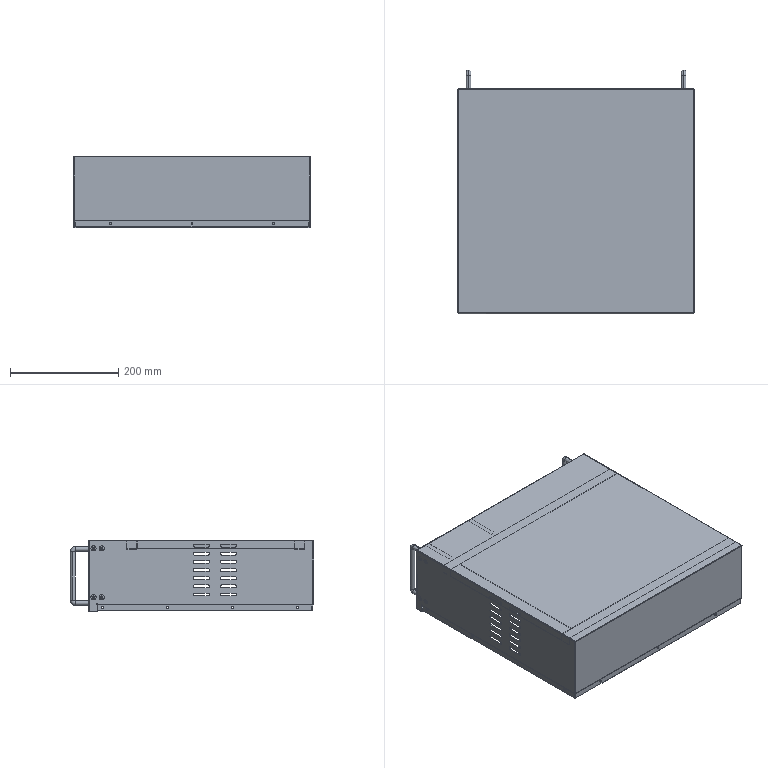Part | SolidWorks | features ICE 25, BossThin 16, LPattern 10, EdgeFlange 7, SMBaseFlange 7, FlatPattern 6, SheetMetal 6, MirrorPattern 4, CornerTrim 2, MirrorSolid 1, Split 1, Sweep 1 | 6 solids | 1057 faces | box 437 x 449.5 x 132 mm | volume 767937 mm3 | cylinder 619 | plane 418 | spline 12 | torus 8 | commonest cylinder face diameters 3.5 x128 4.5 x126 5 x64 5.5 x46 7.5 x40 9.5 x36